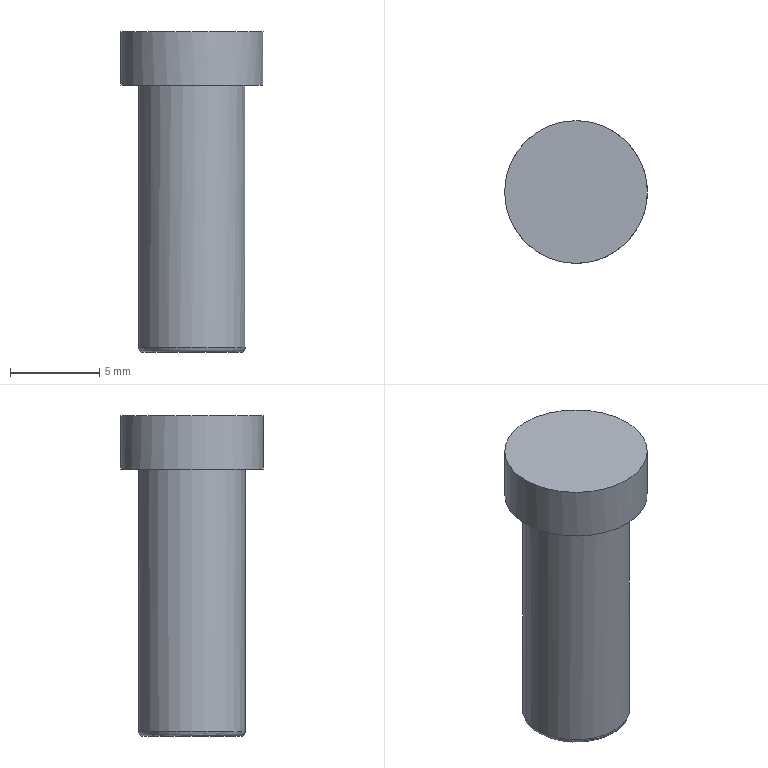Part | STEP file | gslz 2016.10.28-10_id2706_x_t | 1 solid | 6 faces | box 8 x 8 x 18 mm | volume 574.556 mm3 | plane 3 | cylinder 2 | torus 1 | commonest cylinder face diameters 6 x1 8 x1
STEP:
#1=CARTESIAN_POINT('',(0.,0.,0.));
#2=DIRECTION('',(0.,0.,1.));
#3=DIRECTION('',(1.,0.,0.));
#4=AXIS2_PLACEMENT_3D('',#1,#2,#3);
#5=CARTESIAN_POINT('',(-11.,40.,15.));
#6=VERTEX_POINT('',#5);
#7=CARTESIAN_POINT('',(-19.,40.,15.));
#8=VERTEX_POINT('',#7);
#9=CARTESIAN_POINT('',(-15.,40.,15.));
#10=DIRECTION('',(0.,0.,-1.));
#11=DIRECTION('',(1.,0.,0.));
#12=AXIS2_PLACEMENT_3D('',#9,#10,#11);
#13=CIRCLE('',#12,4.);
#14=CARTESIAN_POINT('',(-15.,40.,15.));
#15=DIRECTION('',(0.,0.,1.));
#16=DIRECTION('',(1.,0.,0.));
#17=AXIS2_PLACEMENT_3D('',#14,#15,#16);
#18=PLANE('',#17);
#19=CARTESIAN_POINT('',(4.,0.));
#20=CARTESIAN_POINT('',(4.,-6.928));
#21=CARTESIAN_POINT('',(-2.,-3.464));
#22=CARTESIAN_POINT('',(-8.,0.));
#23=CARTESIAN_POINT('',(-2.,3.464));
#24=CARTESIAN_POINT('',(4.,6.928));
#25=CARTESIAN_POINT('',(4.,0.));
#26=(BOUNDED_CURVE()B_SPLINE_CURVE(2,(#19,#20,#21,#22,#23,#24,#25),.UNSPECIFIED.,.T.,.F.)B_SPLINE_CURVE_WITH_KNOTS((1,2,2,2,2,1),(-2.094,0.,2.094,4.189,6.283,8.378),.UNSPECIFIED.)CURVE()GEOMETRIC_REPRESENTATION_ITEM()RATIONAL_B_SPLINE_CURVE((1.,0.5,1.,0.5,1.,0.5,1.))REPRESENTATION_ITEM(''));
#27=(GEOMETRIC_REPRESENTATION_CONTEXT(2)PARAMETRIC_REPRESENTATION_CONTEXT()REPRESENTATION_CONTEXT('',''));
#28=DEFINITIONAL_REPRESENTATION('',(#26),#27);
#29=PCURVE('',#18,#28);
#30=CARTESIAN_POINT('',(-15.,40.,15.));
#31=DIRECTION('',(0.,0.,-1.));
#32=DIRECTION('',(-1.,0.,0.));
#33=AXIS2_PLACEMENT_3D('',#30,#31,#32);
#34=CYLINDRICAL_SURFACE('',#33,4.);
#35=CARTESIAN_POINT('',(3.142,0.));
#36=DIRECTION('',(1.,0.));
#37=VECTOR('',#36,1.);
#38=LINE('',#35,#37);
#39=(GEOMETRIC_REPRESENTATION_CONTEXT(2)PARAMETRIC_REPRESENTATION_CONTEXT()REPRESENTATION_CONTEXT('',''));
#40=DEFINITIONAL_REPRESENTATION('',(#38),#39);
#41=PCURVE('',#34,#40);
#42=SURFACE_CURVE('',#13,(#29,#41),.PCURVE_S1.);
#43=EDGE_CURVE('',#6,#8,#42,.T.);
#44=ORIENTED_EDGE('',*,*,#43,.F.);
#45=CARTESIAN_POINT('',(-15.,40.,15.));
#46=DIRECTION('',(0.,0.,-1.));
#47=DIRECTION('',(1.,0.,0.));
#48=AXIS2_PLACEMENT_3D('',#45,#46,#47);
#49=CIRCLE('',#48,4.);
#50=CARTESIAN_POINT('',(4.,0.));
#51=CARTESIAN_POINT('',(4.,-6.928));
#52=CARTESIAN_POINT('',(-2.,-3.464));
#53=CARTESIAN_POINT('',(-8.,0.));
#54=CARTESIAN_POINT('',(-2.,3.464));
#55=CARTESIAN_POINT('',(4.,6.928));
#56=CARTESIAN_POINT('',(4.,0.));
#57=(BOUNDED_CURVE()B_SPLINE_CURVE(2,(#50,#51,#52,#53,#54,#55,#56),.UNSPECIFIED.,.T.,.F.)B_SPLINE_CURVE_WITH_KNOTS((1,2,2,2,2,1),(-2.094,0.,2.094,4.189,6.283,8.378),.UNSPECIFIED.)CURVE()GEOMETRIC_REPRESENTATION_ITEM()RATIONAL_B_SPLINE_CURVE((1.,0.5,1.,0.5,1.,0.5,1.))REPRESENTATION_ITEM(''));
#58=(GEOMETRIC_REPRESENTATION_CONTEXT(2)PARAMETRIC_REPRESENTATION_CONTEXT()REPRESENTATION_CONTEXT('',''));
#59=DEFINITIONAL_REPRESENTATION('',(#57),#58);
#60=PCURVE('',#18,#59);
#61=CARTESIAN_POINT('',(-3.142,0.));
#62=DIRECTION('',(1.,0.));
#63=VECTOR('',#62,1.);
#64=LINE('',#61,#63);
#65=(GEOMETRIC_REPRESENTATION_CONTEXT(2)PARAMETRIC_REPRESENTATION_CONTEXT()REPRESENTATION_CONTEXT('',''));
#66=DEFINITIONAL_REPRESENTATION('',(#64),#65);
#67=PCURVE('',#34,#66);
#68=SURFACE_CURVE('',#49,(#60,#67),.PCURVE_S1.);
#69=EDGE_CURVE('',#8,#6,#68,.T.);
#70=ORIENTED_EDGE('',*,*,#69,.F.);
#71=EDGE_LOOP('',(#44,#70));
#72=FACE_BOUND('',#71,.T.);
#73=ADVANCED_FACE('',(#72),#18,.T.);
#74=CARTESIAN_POINT('',(-18.,40.,12.));
#75=VERTEX_POINT('',#74);
#76=CARTESIAN_POINT('',(-15.,40.,12.));
#77=DIRECTION('',(0.,0.,-1.));
#78=DIRECTION('',(-1.,0.,0.));
#79=AXIS2_PLACEMENT_3D('',#76,#77,#78);
#80=CIRCLE('',#79,3.);
#81=CARTESIAN_POINT('',(-15.,40.,12.));
#82=DIRECTION('',(0.,0.,-1.));
#83=DIRECTION('',(-1.,0.,0.));
#84=AXIS2_PLACEMENT_3D('',#81,#82,#83);
#85=PLANE('',#84);
#86=CARTESIAN_POINT('',(0.,0.));
#87=DIRECTION('',(1.,0.));
#88=AXIS2_PLACEMENT_2D('',#86,#87);
#89=CIRCLE('',#88,3.);
#90=(GEOMETRIC_REPRESENTATION_CONTEXT(2)PARAMETRIC_REPRESENTATION_CONTEXT()REPRESENTATION_CONTEXT('',''));
#91=DEFINITIONAL_REPRESENTATION('',(#89),#90);
#92=PCURVE('',#85,#91);
#93=CARTESIAN_POINT('',(-15.,40.,19.));
#94=DIRECTION('',(0.,0.,-1.));
#95=DIRECTION('',(-1.,0.,0.));
#96=AXIS2_PLACEMENT_3D('',#93,#94,#95);
#97=CYLINDRICAL_SURFACE('',#96,3.);
#98=CARTESIAN_POINT('',(0.,7.));
#99=DIRECTION('',(1.,0.));
#100=VECTOR('',#99,1.);
#101=LINE('',#98,#100);
#102=(GEOMETRIC_REPRESENTATION_CONTEXT(2)PARAMETRIC_REPRESENTATION_CONTEXT()REPRESENTATION_CONTEXT('',''));
#103=DEFINITIONAL_REPRESENTATION('',(#101),#102);
#104=PCURVE('',#97,#103);
#105=SURFACE_CURVE('',#80,(#92,#104),.PCURVE_S1.);
#106=EDGE_CURVE('',#75,#75,#105,.T.);
#107=ORIENTED_EDGE('',*,*,#106,.F.);
#108=EDGE_LOOP('',(#107));
#109=FACE_BOUND('',#108,.T.);
#110=CARTESIAN_POINT('',(-19.,40.,12.));
#111=VERTEX_POINT('',#110);
#112=CARTESIAN_POINT('',(-15.,40.,12.));
#113=DIRECTION('',(0.,0.,1.));
#114=DIRECTION('',(-1.,0.,0.));
#115=AXIS2_PLACEMENT_3D('',#112,#113,#114);
#116=CIRCLE('',#115,4.);
#117=CARTESIAN_POINT('',(4.,0.));
#118=CARTESIAN_POINT('',(4.,-6.928));
#119=CARTESIAN_POINT('',(-2.,-3.464));
#120=CARTESIAN_POINT('',(-8.,0.));
#121=CARTESIAN_POINT('',(-2.,3.464));
#122=CARTESIAN_POINT('',(4.,6.928));
#123=CARTESIAN_POINT('',(4.,0.));
#124=(BOUNDED_CURVE()B_SPLINE_CURVE(2,(#117,#118,#119,#120,#121,#122,#123),.UNSPECIFIED.,.T.,.F.)B_SPLINE_CURVE_WITH_KNOTS((1,2,2,2,2,1),(-2.094,0.,2.094,4.189,6.283,8.378),.UNSPECIFIED.)CURVE()GEOMETRIC_REPRESENTATION_ITEM()RATIONAL_B_SPLINE_CURVE((1.,0.5,1.,0.5,1.,0.5,1.))REPRESENTATION_ITEM(''));
#125=(GEOMETRIC_REPRESENTATION_CONTEXT(2)PARAMETRIC_REPRESENTATION_CONTEXT()REPRESENTATION_CONTEXT('',''));
#126=DEFINITIONAL_REPRESENTATION('',(#124),#125);
#127=PCURVE('',#85,#126);
#128=CARTESIAN_POINT('',(6.283,3.));
#129=DIRECTION('',(-1.,0.));
#130=VECTOR('',#129,1.);
#131=LINE('',#128,#130);
#132=(GEOMETRIC_REPRESENTATION_CONTEXT(2)PARAMETRIC_REPRESENTATION_CONTEXT()REPRESENTATION_CONTEXT('',''));
#133=DEFINITIONAL_REPRESENTATION('',(#131),#132);
#134=PCURVE('',#34,#133);
#135=SURFACE_CURVE('',#116,(#127,#134),.PCURVE_S1.);
#136=EDGE_CURVE('',#111,#111,#135,.T.);
#137=ORIENTED_EDGE('',*,*,#136,.F.);
#138=EDGE_LOOP('',(#137));
#139=FACE_BOUND('',#138,.T.);
#140=ADVANCED_FACE('',(#109,#139),#85,.T.);
#141=ORIENTED_EDGE('',*,*,#136,.T.);
#142=CARTESIAN_POINT('',(-19.,40.,15.));
#143=CARTESIAN_POINT('',(-19.,40.,12.));
#144=B_SPLINE_CURVE_WITH_KNOTS('',1,(#142,#143),.UNSPECIFIED.,.F.,.F.,(2,2),(0.,3.),.PIECEWISE_BEZIER_KNOTS.);
#145=CARTESIAN_POINT('',(0.,0.));
#146=DIRECTION('',(0.,1.));
#147=VECTOR('',#146,1.);
#148=LINE('',#145,#147);
#149=(GEOMETRIC_REPRESENTATION_CONTEXT(2)PARAMETRIC_REPRESENTATION_CONTEXT()REPRESENTATION_CONTEXT('',''));
#150=DEFINITIONAL_REPRESENTATION('',(#148),#149);
#151=PCURVE('',#34,#150);
#152=CARTESIAN_POINT('',(6.283,0.));
#153=DIRECTION('',(0.,1.));
#154=VECTOR('',#153,1.);
#155=LINE('',#152,#154);
#156=(GEOMETRIC_REPRESENTATION_CONTEXT(2)PARAMETRIC_REPRESENTATION_CONTEXT()REPRESENTATION_CONTEXT('',''));
#157=DEFINITIONAL_REPRESENTATION('',(#155),#156);
#158=PCURVE('',#34,#157);
#159=SEAM_CURVE('',#144,(#151,#158),.PCURVE_S1.);
#160=EDGE_CURVE('',#8,#111,#159,.T.);
#161=ORIENTED_EDGE('',*,*,#160,.F.);
#162=ORIENTED_EDGE('',*,*,#69,.T.);
#163=ORIENTED_EDGE('',*,*,#43,.T.);
#164=ORIENTED_EDGE('',*,*,#160,.T.);
#165=EDGE_LOOP('',(#141,#161,#162,#163,#164));
#166=FACE_BOUND('',#165,.T.);
#167=ADVANCED_FACE('',(#166),#34,.T.);
#168=CARTESIAN_POINT('',(-12.3,40.,-3.));
#169=VERTEX_POINT('',#168);
#170=CARTESIAN_POINT('',(-15.,40.,-3.));
#171=DIRECTION('',(0.,0.,-1.));
#172=DIRECTION('',(-1.,0.,0.));
#173=AXIS2_PLACEMENT_3D('',#170,#171,#172);
#174=CIRCLE('',#173,2.7);
#175=CARTESIAN_POINT('',(-15.,40.,-3.));
#176=DIRECTION('',(0.,0.,-1.));
#177=DIRECTION('',(-1.,0.,0.));
#178=AXIS2_PLACEMENT_3D('',#175,#176,#177);
#179=PLANE('',#178);
#180=CARTESIAN_POINT('',(0.,0.));
#181=DIRECTION('',(1.,0.));
#182=AXIS2_PLACEMENT_2D('',#180,#181);
#183=CIRCLE('',#182,2.7);
#184=(GEOMETRIC_REPRESENTATION_CONTEXT(2)PARAMETRIC_REPRESENTATION_CONTEXT()REPRESENTATION_CONTEXT('',''));
#185=DEFINITIONAL_REPRESENTATION('',(#183),#184);
#186=PCURVE('',#179,#185);
#187=CARTESIAN_POINT('',(-15.,40.,-2.7));
#188=DIRECTION('',(0.,0.,-1.));
#189=DIRECTION('',(1.,0.,0.));
#190=AXIS2_PLACEMENT_3D('',#187,#188,#189);
#191=TOROIDAL_SURFACE('',#190,2.7,0.3);
#192=CARTESIAN_POINT('',(-3.142,7.854));
#193=DIRECTION('',(1.,0.));
#194=VECTOR('',#193,1.);
#195=LINE('',#192,#194);
#196=(GEOMETRIC_REPRESENTATION_CONTEXT(2)PARAMETRIC_REPRESENTATION_CONTEXT()REPRESENTATION_CONTEXT('',''));
#197=DEFINITIONAL_REPRESENTATION('',(#195),#196);
#198=PCURVE('',#191,#197);
#199=SURFACE_CURVE('',#174,(#186,#198),.PCURVE_S1.);
#200=EDGE_CURVE('',#169,#169,#199,.T.);
#201=ORIENTED_EDGE('',*,*,#200,.T.);
#202=EDGE_LOOP('',(#201));
#203=FACE_BOUND('',#202,.T.);
#204=ADVANCED_FACE('',(#203),#179,.T.);
#205=CARTESIAN_POINT('',(-18.,40.,-2.7));
#206=VERTEX_POINT('',#205);
#207=CARTESIAN_POINT('',(-12.,40.,-2.7));
#208=VERTEX_POINT('',#207);
#209=CARTESIAN_POINT('',(-15.,40.,-2.7));
#210=DIRECTION('',(0.,0.,1.));
#211=DIRECTION('',(-1.,0.,0.));
#212=AXIS2_PLACEMENT_3D('',#209,#210,#211);
#213=CIRCLE('',#212,3.);
#214=CARTESIAN_POINT('',(6.283,21.7));
#215=DIRECTION('',(-1.,0.));
#216=VECTOR('',#215,1.);
#217=LINE('',#214,#216);
#218=(GEOMETRIC_REPRESENTATION_CONTEXT(2)PARAMETRIC_REPRESENTATION_CONTEXT()REPRESENTATION_CONTEXT('',''));
#219=DEFINITIONAL_REPRESENTATION('',(#217),#218);
#220=PCURVE('',#97,#219);
#221=CARTESIAN_POINT('',(3.142,6.283));
#222=DIRECTION('',(-1.,0.));
#223=VECTOR('',#222,1.);
#224=LINE('',#221,#223);
#225=(GEOMETRIC_REPRESENTATION_CONTEXT(2)PARAMETRIC_REPRESENTATION_CONTEXT()REPRESENTATION_CONTEXT('',''));
#226=DEFINITIONAL_REPRESENTATION('',(#224),#225);
#227=PCURVE('',#191,#226);
#228=SURFACE_CURVE('',#213,(#220,#227),.PCURVE_S1.);
#229=EDGE_CURVE('',#206,#208,#228,.T.);
#230=ORIENTED_EDGE('',*,*,#229,.T.);
#231=CARTESIAN_POINT('',(-15.,40.,-2.7));
#232=DIRECTION('',(0.,0.,1.));
#233=DIRECTION('',(-1.,0.,0.));
#234=AXIS2_PLACEMENT_3D('',#231,#232,#233);
#235=CIRCLE('',#234,3.);
#236=CARTESIAN_POINT('',(6.283,21.7));
#237=DIRECTION('',(-1.,0.));
#238=VECTOR('',#237,1.);
#239=LINE('',#236,#238);
#240=(GEOMETRIC_REPRESENTATION_CONTEXT(2)PARAMETRIC_REPRESENTATION_CONTEXT()REPRESENTATION_CONTEXT('',''));
#241=DEFINITIONAL_REPRESENTATION('',(#239),#240);
#242=PCURVE('',#97,#241);
#243=CARTESIAN_POINT('',(9.425,6.283));
#244=DIRECTION('',(-1.,0.));
#245=VECTOR('',#244,1.);
#246=LINE('',#243,#245);
#247=(GEOMETRIC_REPRESENTATION_CONTEXT(2)PARAMETRIC_REPRESENTATION_CONTEXT()REPRESENTATION_CONTEXT('',''));
#248=DEFINITIONAL_REPRESENTATION('',(#246),#247);
#249=PCURVE('',#191,#248);
#250=SURFACE_CURVE('',#235,(#242,#249),.PCURVE_S1.);
#251=EDGE_CURVE('',#208,#206,#250,.T.);
#252=ORIENTED_EDGE('',*,*,#251,.T.);
#253=CARTESIAN_POINT('',(-18.,40.,12.));
#254=CARTESIAN_POINT('',(-18.,40.,-2.7));
#255=B_SPLINE_CURVE_WITH_KNOTS('',1,(#253,#254),.UNSPECIFIED.,.F.,.F.,(2,2),(7.,21.7),.PIECEWISE_BEZIER_KNOTS.);
#256=CARTESIAN_POINT('',(0.,0.));
#257=DIRECTION('',(0.,1.));
#258=VECTOR('',#257,1.);
#259=LINE('',#256,#258);
#260=(GEOMETRIC_REPRESENTATION_CONTEXT(2)PARAMETRIC_REPRESENTATION_CONTEXT()REPRESENTATION_CONTEXT('',''));
#261=DEFINITIONAL_REPRESENTATION('',(#259),#260);
#262=PCURVE('',#97,#261);
#263=CARTESIAN_POINT('',(6.283,0.));
#264=DIRECTION('',(0.,1.));
#265=VECTOR('',#264,1.);
#266=LINE('',#263,#265);
#267=(GEOMETRIC_REPRESENTATION_CONTEXT(2)PARAMETRIC_REPRESENTATION_CONTEXT()REPRESENTATION_CONTEXT('',''));
#268=DEFINITIONAL_REPRESENTATION('',(#266),#267);
#269=PCURVE('',#97,#268);
#270=SEAM_CURVE('',#255,(#262,#269),.PCURVE_S1.);
#271=EDGE_CURVE('',#75,#206,#270,.T.);
#272=ORIENTED_EDGE('',*,*,#271,.F.);
#273=ORIENTED_EDGE('',*,*,#106,.T.);
#274=ORIENTED_EDGE('',*,*,#271,.T.);
#275=EDGE_LOOP('',(#230,#252,#272,#273,#274));
#276=FACE_BOUND('',#275,.T.);
#277=ADVANCED_FACE('',(#276),#97,.T.);
#278=ORIENTED_EDGE('',*,*,#200,.F.);
#279=CARTESIAN_POINT('',(-12.,40.,-2.7));
#280=CARTESIAN_POINT('',(-12.,40.,-2.78));
#281=CARTESIAN_POINT('',(-12.026,40.,-2.858));
#282=CARTESIAN_POINT('',(-12.074,40.,-2.926));
#283=CARTESIAN_POINT('',(-12.142,40.,-2.974));
#284=CARTESIAN_POINT('',(-12.22,40.,-3.));
#285=CARTESIAN_POINT('',(-12.3,40.,-3.));
#286=(BOUNDED_CURVE()B_SPLINE_CURVE(6,(#279,#280,#281,#282,#283,#284,#285),.UNSPECIFIED.,.F.,.F.)B_SPLINE_CURVE_WITH_KNOTS((7,7),(0.,1.571),.PIECEWISE_BEZIER_KNOTS.)CURVE()GEOMETRIC_REPRESENTATION_ITEM()RATIONAL_B_SPLINE_CURVE((1.031,1.01,0.9979,0.994,0.9979,1.01,1.031))REPRESENTATION_ITEM(''));
#287=CARTESIAN_POINT('',(0.,6.283));
#288=DIRECTION('',(0.,1.));
#289=VECTOR('',#288,1.);
#290=LINE('',#287,#289);
#291=(GEOMETRIC_REPRESENTATION_CONTEXT(2)PARAMETRIC_REPRESENTATION_CONTEXT()REPRESENTATION_CONTEXT('',''));
#292=DEFINITIONAL_REPRESENTATION('',(#290),#291);
#293=PCURVE('',#191,#292);
#294=CARTESIAN_POINT('',(6.283,6.283));
#295=DIRECTION('',(0.,1.));
#296=VECTOR('',#295,1.);
#297=LINE('',#294,#296);
#298=(GEOMETRIC_REPRESENTATION_CONTEXT(2)PARAMETRIC_REPRESENTATION_CONTEXT()REPRESENTATION_CONTEXT('',''));
#299=DEFINITIONAL_REPRESENTATION('',(#297),#298);
#300=PCURVE('',#191,#299);
#301=SEAM_CURVE('',#286,(#293,#300),.PCURVE_S1.);
#302=EDGE_CURVE('',#208,#169,#301,.T.);
#303=ORIENTED_EDGE('',*,*,#302,.F.);
#304=ORIENTED_EDGE('',*,*,#229,.F.);
#305=ORIENTED_EDGE('',*,*,#251,.F.);
#306=ORIENTED_EDGE('',*,*,#302,.T.);
#307=EDGE_LOOP('',(#278,#303,#304,#305,#306));
#308=FACE_BOUND('',#307,.T.);
#309=ADVANCED_FACE('',(#308),#191,.T.);
#310=CLOSED_SHELL('',(#73,#140,#167,#204,#277,#309));
#311=MANIFOLD_SOLID_BREP('',#310);
#312=(LENGTH_UNIT()NAMED_UNIT(*)SI_UNIT(.MILLI.,.METRE.));
#313=UNCERTAINTY_MEASURE_WITH_UNIT(LENGTH_MEASURE(0.000005),#312,'','');
#314=(NAMED_UNIT(*)PLANE_ANGLE_UNIT()SI_UNIT($,.RADIAN.));
#315=(NAMED_UNIT(*)SI_UNIT($,.STERADIAN.)SOLID_ANGLE_UNIT());
#316=(GEOMETRIC_REPRESENTATION_CONTEXT(3)GLOBAL_UNCERTAINTY_ASSIGNED_CONTEXT((#313))GLOBAL_UNIT_ASSIGNED_CONTEXT((#312,#314,#315))REPRESENTATION_CONTEXT('',''));
#317=ADVANCED_BREP_SHAPE_REPRESENTATION('',(#4,#311),#316);